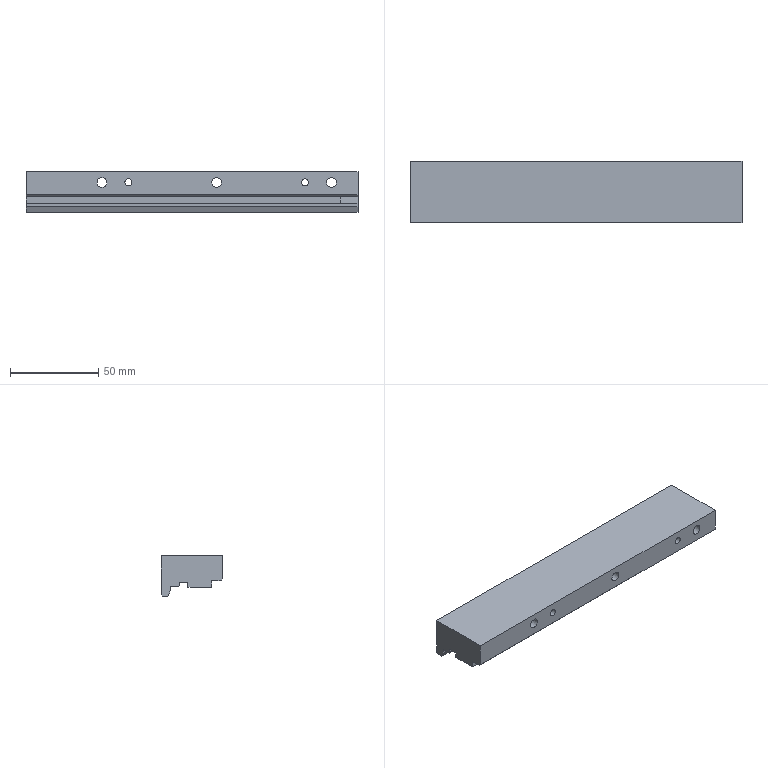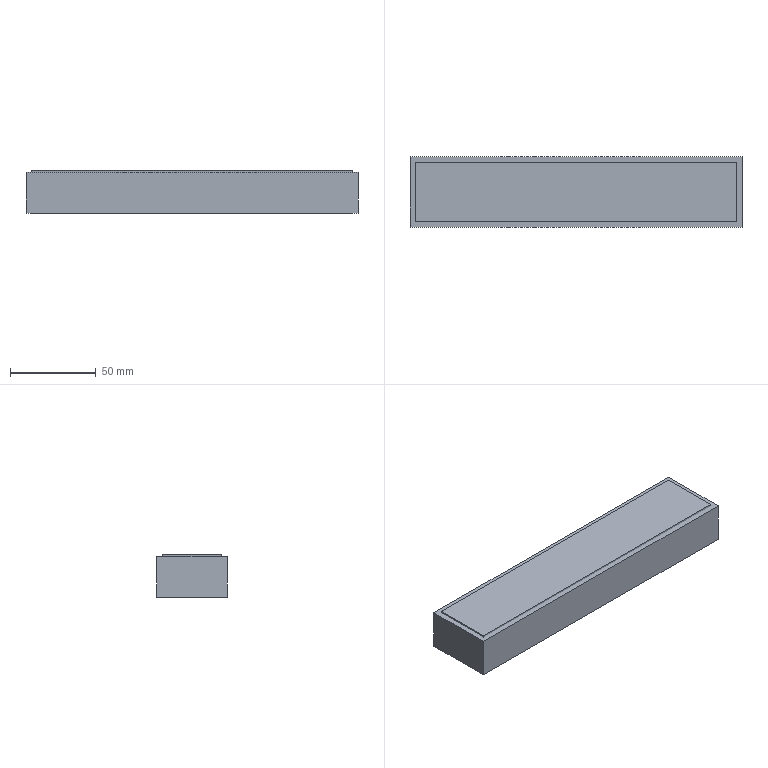CAM job | NX | 3-axis milling | part box 188 x 35 x 22.9 mm | stock box 194 x 41 x 24.9 mm
Tools:
number,name,description,diameter,corner_radius,flute_length,length,flutes
1,D50,Milling Tool-5 Parameters,50.0,0.0,50.0,75.0,2
3,D10,Milling Tool-5 Parameters,10.0,0.0,50.0,75.0,2
4,D10JING,Milling Tool-5 Parameters,10.0,0.0,50.0,75.0,2
2,D6A45,Milling Tool-5 Parameters,6.0,0.0,3.0,3.0,2
8,D6,Milling Tool-5 Parameters,6.0,0.0,50.0,75.0,2
10,D4,Milling Tool-5 Parameters,4.0,0.0,50.0,75.0,2
20,D6R0.5,Milling Tool-5 Parameters,6.0,0.5,50.0,75.0,2
Operations:
program,operation,operation_type,tool,method,geometry_group,spindle_rpm,surface_speed,feed_per_tooth,feed_cut,feed_plunge,cut_length_mm,path_length_mm,cut_time_min,machine_time_min
1-193-40-25毛胚,FLOOR_WALL,VolumeBased25DMillingOperation,D50,METHOD,A,6500.0,1286.0,0.0962,1250.0,100.0,256.0,310.0,0.2048,0.2102
1-193-40-25毛胚,ZLEVEL_PROFILE,ZLevelMilling,D10,METHOD,A,7000.0,219.0,0.2143,3000.0,1000.0,11101.435,11181.335,3.732,3.74
1-193-40-25毛胚,ZLEVEL_PROFILE_COPY_COPY_1_COPY_COPY_COPY_1,ZLevelMilling,D10JING,METHOD,A,7000.0,219.0,0.0714,1000.0,100.0,961.097,1067.116,0.9611,0.9717
1-193-40-25毛胚,ZLEVEL_PROFILE_COPY_1_COPY_COPY_COPY_COPY_2_COPY,ZLevelMilling,D6A45,METHOD,A,7000.0,131.0,0.0714,1000.0,1000.0,455.121,517.121,0.4551,0.4613
2-193-40-25毛胚,FLOOR_WALL_COPY,VolumeBased25DMillingOperation,D50,METHOD,B,6500.0,1286.0,0.0962,1250.0,100.0,500.0,850,0.4,0.435
2-193-40-25毛胚,FLOOR_WALL_1,VolumeBased25DMillingOperation,D10,METHOD,B,7000.0,219.0,0.2143,3000.0,1000.0,1441.035,1771.567,0.49,0.5231
2-193-40-25毛胚,FLOOR_WALL_1_COPY,VolumeBased25DMillingOperation,D10,METHOD,B,7000.0,219.0,0.2143,3000.0,1000.0,4770.947,4834.647,1.596,1.602
2-193-40-25毛胚,FLOOR_WALL_1_COPY_1_1,VolumeBased25DMillingOperation,D6,METHOD,B,7000.0,87.0,0.0714,1000.0,100.0,2411.41,2635.107,2.411,2.434
2-193-40-25毛胚,FLOOR_WALL_1_1,VolumeBased25DMillingOperation,D4,METHOD,B,7000.0,87.0,0.1429,2000.0,1000.0,2727.9,2801.6,1.385,1.393
2-193-40-25毛胚,FLOOR_WALL_1_COPY_1,VolumeBased25DMillingOperation,D4,METHOD,B,7000.0,87.0,0.0714,1000.0,100.0,793.599,869.999,0.7936,0.8013
2-193-40-25毛胚,ZLEVEL_PROFILE_COPY_COPY_1_COPY_COPY_COPY_1_COPY_COPY,ZLevelMilling,D6R0.5,METHOD,B,7000.0,131.0,0.2143,3000.0,1000.0,7374.417,7438.007,2.459,2.465
2-193-40-25毛胚,ZLEVEL_PROFILE_COPY_1_COPY_COPY_COPY_COPY_2_COPY_COPY_COPY_COPY,ZLevelMilling,D6A45,METHOD,B,7000.0,131.0,0.0714,1000.0,1000.0,208.649,271.649,0.2086,0.2149
2-193-40-25毛胚,ZLEVEL_PROFILE_COPY_1_COPY_COPY_COPY_COPY_2_COPY_COPY,ZLevelMilling,D6A45,METHOD,B,7000.0,131.0,0.0714,1000.0,1000.0,611.125,949.672,0.6111,0.645
2-193-40-25毛胚,ZLEVEL_PROFILE_COPY_1_COPY_COPY_COPY_COPY_2_COPY_COPY_COPY,ZLevelMilling,D6A45,METHOD,B,7000.0,131.0,0.0714,1000.0,1000.0,206.664,288.264,0.2067,0.2148